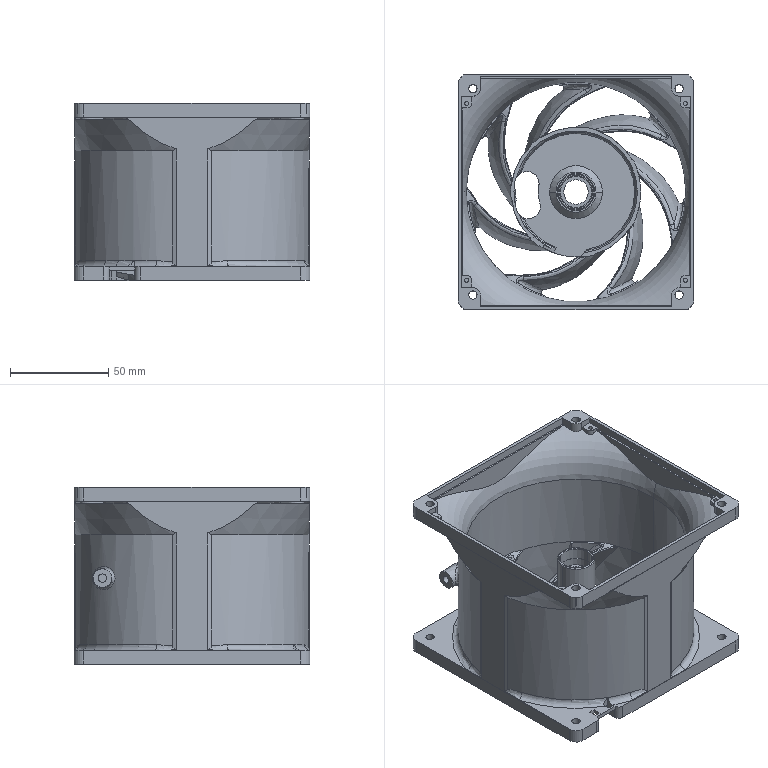NC program | NX | posted with a generic post | part box 120 x 120 x 90.2 mm
Lines 89761 to 90543 of 941997:
(QUICK_ROUGHING , TOOL : D8开粗刀)
N179490 T03 M6
N179492 G54
N179494 G17 G0 G90 X-40.033 Y2.81 S6800 M3
N179496 G43 Z3.6 H3
N179498 Z-0.8
N179500 G94 G1 Z-1.3 F2500.
N179502 G3 X-36.653 Y5.989 R4.
N179504 G2 X-34.912 Y12.669 R43.674
N179506 G3 X-34.604 Y14.896 R51.775
N179508 G2 X-33.059 Y17.237 R5.097
N179510 G3 X-32.058 Y18.68 R7.307
N179512 G1 X-30.488 Y21.219
N179514 G2 X-24.92 Y27.542 R44.968
N179516 X-18.509 Y32.196 R43.58
N179518 X-11.865 Y35.2 R44.159
N179520 G3 X-10.38 Y36.109 R8.325
N179522 G2 X-7.101 Y36.597 R4.998
N179524 G3 X-3.264 Y36.97 R28.124
N179526 X-2.561 Y38.44 R0.967
N179528 G1 X-3.523 Y39.986
N179530 Z-0.8
N179532 G0 Z0.7
N179534 X-3.52 Z0.77
N179536 X-3.511 Z0.839
N179538 X-3.496 Y39.987 Z0.907
N179540 X-3.475 Y39.988 Z0.974
N179542 X-3.449 Y39.989 Z1.038
N179544 X-3.416 Y39.99 Z1.1
N179546 X-3.379 Y39.992 Z1.159
N179548 X-3.336 Y39.994 Z1.214
N179550 X-3.289 Y39.996 Z1.266
N179552 X-3.238 Y39.998 Z1.313
N179554 X-3.183 Y40. Z1.355
N179556 X-3.124 Y40.003 Z1.393
N179558 X-3.062 Y40.005 Z1.425
N179560 X-2.997 Y40.008 Z1.452
N179562 X-2.931 Y40.011 Z1.473
N179564 X-2.863 Y40.014 Z1.488
N179566 X-2.794 Y40.016 Z1.497
N179568 X-2.724 Y40.019 Z1.5
N179570 X-0.994 Y40.092
N179572 X-0.925 Y40.095 Z1.497
N179574 X-0.856 Y40.098 Z1.488
N179576 X-0.787 Y40.101 Z1.473
N179578 X-0.721 Y40.104 Z1.452
N179580 X-0.657 Y40.106 Z1.425
N179582 X-0.595 Y40.109 Z1.393
N179584 X-0.536 Y40.111 Z1.355
N179586 X-0.481 Y40.114 Z1.313
N179588 X-0.429 Y40.116 Z1.266
N179590 X-0.382 Y40.118 Z1.214
N179592 X-0.34 Y40.12 Z1.159
N179594 X-0.302 Y40.121 Z1.1
N179596 X-0.27 Y40.123 Z1.038
N179598 X-0.243 Y40.124 Z0.974
N179600 X-0.222 Y40.125 Z0.907
N179602 X-0.207 Z0.839
N179604 X-0.198 Y40.126 Z0.77
N179606 X-0.195 Z0.7
N179608 Z-0.8
N179610 G1 Z-1.3
N179612 G3 X3.232 Y36.973 R4.
N179614 G2 X19.426 Y31.636 R37.113
N179616 G3 X21.232 Y30.792 R5.732
N179618 G2 X23.894 Y28.827 R4.47
N179620 G3 X25.83 Y26.638 R15.265
N179622 G2 X32.163 Y18.509 R36.014
N179624 G1 X32.706 Y17.606
N179626 X34.407 Y13.993
N179628 G2 X36.951 Y3.715 R41.082
N179630 G3 X37.49 Y2.165 R7.171
N179632 G2 X37.271 Y-1.201 R5.018
N179634 G3 X36.981 Y-3.168 R9.676
N179636 G2 X32.669 Y-17.62 R37.115
N179638 X25.935 Y-26.599 R38.992
N179640 G1 X24.695 Y-28.458
N179642 G2 X22.235 Y-29.913 R5.67
N179644 G3 X20.329 Y-31.043 R16.913
N179646 G2 X14.91 Y-33.978 R31.887
N179648 X13.103 Y-34.723 R10.108
N179650 X6.324 Y-36.587 R39.685
N179652 X-4.182 Y-36.893 R38.958
N179654 G3 X-6.767 Y-37.051 R16.229
N179656 G2 X-9.477 Y-36.037 R5.102
N179658 G1 X-9.735 Y-35.926
N179660 G3 X-11.169 Y-36.84 R1.026
N179662 G1 X-11.214 Y-38.581
N179664 Z-0.8
N179666 G0 Z-0.1
N179668 X-11.211 Y-38.583 Z-0.03
N179670 X-11.204 Y-38.588 Z0.039
N179672 X-11.191 Y-38.596 Z0.107
N179674 X-11.173 Y-38.607 Z0.174
N179676 X-11.151 Y-38.622 Z0.238
N179678 X-11.123 Y-38.639 Z0.3
N179680 X-11.092 Y-38.659 Z0.359
N179682 X-11.056 Y-38.682 Z0.414
N179684 X-11.016 Y-38.707 Z0.466
N179686 X-10.973 Y-38.734 Z0.513
N179688 X-10.926 Y-38.764 Z0.555
N179690 X-10.876 Y-38.796 Z0.593
N179692 X-10.824 Y-38.829 Z0.625
N179694 X-10.769 Y-38.863 Z0.652
N179696 X-10.713 Y-38.899 Z0.673
N179698 X-10.656 Y-38.935 Z0.688
N179700 X-10.597 Y-38.973 Z0.697
N179702 X-10.538 Y-39.01 Z0.7
N179704 X-1.277 Y-44.885
N179706 X-1.218 Y-44.922 Z0.697
N179708 X-1.159 Y-44.959 Z0.688
N179710 X-1.102 Y-44.996 Z0.673
N179712 X-1.046 Y-45.032 Z0.652
N179714 X-0.991 Y-45.066 Z0.625
N179716 X-0.939 Y-45.099 Z0.593
N179718 X-0.889 Y-45.131 Z0.555
N179720 X-0.842 Y-45.16 Z0.513
N179722 X-0.799 Y-45.188 Z0.466
N179724 X-0.759 Y-45.213 Z0.414
N179726 X-0.723 Y-45.236 Z0.359
N179728 X-0.692 Y-45.256 Z0.3
N179730 X-0.664 Y-45.273 Z0.238
N179732 X-0.642 Y-45.288 Z0.174
N179734 X-0.624 Y-45.299 Z0.107
N179736 X-0.611 Y-45.307 Z0.039
N179738 X-0.604 Y-45.312 Z-0.03
N179740 X-0.601 Y-45.314 Z-0.1
N179742 Z-1.6
N179744 G1 Z-2.1
N179746 G2 X1.532 Y-42.648 R4.
N179748 G3 X3.574 Y-41.161 R9.885
N179750 G2 X4.475 Y-40.84 R2.049
N179752 G1 X5.731 Y-40.696
N179754 G2 X7.956 Y-42.7 R1.998
N179756 G1 Z-1.6
N179758 G0 X7.959 Y-42.698 Z-1.53
N179760 X7.967 Y-42.693 Z-1.461
N179762 X7.98 Y-42.686 Z-1.393
N179764 X7.998 Y-42.675 Z-1.326
N179766 X8.021 Y-42.662 Z-1.262
N179768 X8.048 Y-42.645 Z-1.2
N179770 X8.081 Y-42.626 Z-1.141
N179772 X8.117 Y-42.605 Z-1.086
N179774 X8.158 Y-42.581 Z-1.034
N179776 X8.202 Y-42.555 Z-0.987
N179778 X8.25 Y-42.527 Z-0.945
N179780 X8.301 Y-42.497 Z-0.907
N179782 X8.354 Y-42.465 Z-0.875
N179784 X8.41 Y-42.433 Z-0.848
N179786 X8.467 Y-42.399 Z-0.827
N179788 X8.526 Y-42.364 Z-0.812
N179790 X8.586 Y-42.329 Z-0.803
N179792 X8.646 Y-42.294 Z-0.8
N179794 X25.242 Y-32.533
N179796 X25.302 Y-32.498 Z-0.803
N179798 X25.362 Y-32.463 Z-0.812
N179800 X25.42 Y-32.428 Z-0.827
N179802 X25.478 Y-32.394 Z-0.848
N179804 X25.533 Y-32.362 Z-0.875
N179806 X25.587 Y-32.33 Z-0.907
N179808 X25.637 Y-32.301 Z-0.945
N179810 X25.685 Y-32.273 Z-0.987
N179812 X25.73 Y-32.246 Z-1.034
N179814 X25.77 Y-32.223 Z-1.086
N179816 X25.807 Y-32.201 Z-1.141
N179818 X25.839 Y-32.182 Z-1.2
N179820 X25.867 Y-32.166 Z-1.262
N179822 X25.89 Y-32.152 Z-1.326
N179824 X25.908 Y-32.141 Z-1.393
N179826 X25.921 Y-32.134 Z-1.461
N179828 X25.929 Y-32.129 Z-1.53
N179830 X25.932 Y-32.128 Z-1.6
N179832 G1 Z-2.1
N179834 G3 X20.48 Y-30.949 R4.
N179836 G1 X17.62 Y-32.699
N179838 X14.007 Y-34.402
N179840 G2 X5.878 Y-36.676 R43.391
N179842 G3 X1.968 Y-37.13 R56.548
N179844 X1.172 Y-37.742 R1.737
N179846 G2 X-1.348 Y-39.543 R4.107
N179848 X-5.71 Y-38.922 R4.778
N179850 G3 X-7.2 Y-39.648 R0.99
N179852 G1 X-7.425 Y-41.417
N179854 Z-1.6
N179856 G0 Z0.7
N179858 X-7.428 Y-41.416 Z0.77
N179860 X-7.436 Y-41.411 Z0.839
N179862 X-7.448 Y-41.402 Z0.907
N179864 X-7.466 Y-41.391 Z0.974
N179866 X-7.488 Y-41.377 Z1.038
N179868 X-7.515 Y-41.359 Z1.1
N179870 X-7.547 Y-41.339 Z1.159
N179872 X-7.583 Y-41.316 Z1.214
N179874 X-7.623 Y-41.291 Z1.266
N179876 X-7.666 Y-41.263 Z1.313
N179878 X-7.712 Y-41.233 Z1.355
N179880 X-7.762 Y-41.201 Z1.393
N179882 X-7.814 Y-41.168 Z1.425
N179884 X-7.868 Y-41.133 Z1.452
N179886 X-7.924 Y-41.097 Z1.473
N179888 X-7.982 Y-41.06 Z1.488
N179890 X-8.04 Y-41.023 Z1.497
N179892 X-8.099 Y-40.985 Z1.5
N179894 X-11.885 Y-38.557
N179896 X-11.944 Y-38.52 Z1.497
N179898 X-12.002 Y-38.482 Z1.488
N179900 X-12.06 Y-38.445 Z1.473
N179902 X-12.116 Y-38.409 Z1.452
N179904 X-12.17 Y-38.375 Z1.425
N179906 X-12.222 Y-38.341 Z1.393
N179908 X-12.272 Y-38.309 Z1.355
N179910 X-12.318 Y-38.28 Z1.313
N179912 X-12.362 Y-38.252 Z1.266
N179914 X-12.401 Y-38.226 Z1.214
N179916 X-12.437 Y-38.203 Z1.159
N179918 X-12.469 Y-38.183 Z1.1
N179920 X-12.496 Y-38.166 Z1.038
N179922 X-12.518 Y-38.151 Z0.974
N179924 X-12.536 Y-38.14 Z0.907
N179926 X-12.549 Y-38.132 Z0.839
N179928 X-12.556 Y-38.127 Z0.77
N179930 X-12.559 Y-38.125 Z0.7
N179932 Z-0.8
N179934 G1 Z-1.3
N179936 G3 X-14.825 Y-34.015 R4.
N179938 G2 X-18.659 Y-32.071 R29.796
N179940 X-23.929 Y-28.374 R35.194
N179942 X-31.503 Y-19.655 R37.735
N179944 G3 X-32.961 Y-18.09 R7.299
N179946 G2 X-34.078 Y-15.232 R4.788
N179948 G3 X-34.647 Y-13.271 R8.83
N179950 G2 X-36.957 Y-3.368 R35.846
N179952 G3 X-38.424 Y-2.67 R0.963
N179954 G1 X-39.972 Y-3.639
N179956 Z-0.8
N179958 G0 Z-0.1
N179960 X-39.973 Y-3.637 Z-0.03
N179962 X-39.978 Y-3.629 Z0.039
N179964 X-39.985 Y-3.615 Z0.107
N179966 X-39.995 Y-3.597 Z0.174
N179968 X-40.009 Y-3.574 Z0.238
N179970 X-40.025 Y-3.546 Z0.3
N179972 X-40.043 Y-3.513 Z0.359
N179974 X-40.064 Y-3.476 Z0.414
N179976 X-40.087 Y-3.435 Z0.466
N179978 X-40.113 Y-3.391 Z0.513
N179980 X-40.14 Y-3.343 Z0.555
N179982 X-40.169 Y-3.291 Z0.593
N179984 X-40.2 Y-3.238 Z0.625
N179986 X-40.232 Y-3.182 Z0.652
N179988 X-40.265 Y-3.124 Z0.673
N179990 X-40.298 Y-3.065 Z0.688
N179992 X-40.332 Y-3.004 Z0.697
N179994 X-40.367 Y-2.944 Z0.7
N179996 X-42.04 Y-0.001
N179998 X-42.075 Y0.06 Z0.697
N180000 X-42.109 Y0.12 Z0.688
N180002 X-42.142 Y0.179 Z0.673
N180004 X-42.175 Y0.237 Z0.652
N180006 X-42.207 Y0.293 Z0.625
N180008 X-42.238 Y0.347 Z0.593
N180010 X-42.267 Y0.398 Z0.555
N180012 X-42.294 Y0.446 Z0.513
N180014 X-42.32 Y0.491 Z0.466
N180016 X-42.343 Y0.532 Z0.414
N180018 X-42.364 Y0.569 Z0.359
N180020 X-42.383 Y0.601 Z0.3
N180022 X-42.399 Y0.629 Z0.238
N180024 X-42.412 Y0.652 Z0.174
N180026 X-42.422 Y0.671 Z0.107
N180028 X-42.43 Y0.684 Z0.039
N180030 X-42.434 Y0.692 Z-0.03
N180032 X-42.436 Y0.694 Z-0.1
N180034 Z-1.6
N180036 G1 Z-2.1
N180038 G3 X-40.949 Y3.424 R4.
N180040 X-40.868 Y5.466 R7.112
N180042 X-41.624 Y7.158 R24.03
N180044 G1 X-41.917 Y8.015
N180046 G3 X-44.85 Y8.618 R1.733
N180048 G2 X-45.422 Y8.249 R1.068
N180050 X-45.389 Y8.753 R0.531
N180052 X-42.313 Y14.072 R28.836
N180054 X-38.596 Y18.485 R25.146
N180056 X-36.867 Y19.406 R3.238
N180058 X-36.002 Y18.772 R0.918
N180060 X-36.756 Y14.155 R4.
N180062 G3 X-38.26 Y10.38 R4.599
N180064 X-37.455 Y7.671 R4.506
N180066 G2 X-36.631 Y6.282 R1.957
N180068 G3 X-37.071 Y-2.265 R44.612
N180070 G1 X-36.514 Y-6.781
N180072 X-35.854 Y-9.557
N180074 G2 X-36.983 Y-10.706 R0.952
N180076 G1 X-38.785 Y-10.313
N180078 Z-1.6
N180080 G0 Z0.198
N180082 Y-10.315 Z0.242
N180084 X-38.783 Y-10.32 Z0.285
N180086 X-38.781 Y-10.329 Z0.328
N180088 X-38.777 Y-10.342 Z0.37
N180090 X-38.773 Y-10.358 Z0.41
N180092 X-38.767 Y-10.378 Z0.449
N180094 X-38.761 Y-10.4 Z0.486
N180096 X-38.754 Y-10.426 Z0.521
N180098 X-38.746 Y-10.455 Z0.553
N180100 X-38.737 Y-10.486 Z0.583
N180102 X-38.728 Y-10.519 Z0.609
N180104 X-38.718 Y-10.555 Z0.633
N180106 X-38.707 Y-10.592 Z0.653
N180108 X-38.697 Y-10.631 Z0.67
N180110 X-38.685 Y-10.671 Z0.683
N180112 X-38.674 Y-10.713 Z0.692
N180114 X-38.662 Y-10.754 Z0.698
N180116 X-38.65 Y-10.797 Z0.7
N180118 X-38.639 Y-10.839 Z0.698
N180120 X-38.627 Y-10.881 Z0.692
N180122 X-38.615 Y-10.922 Z0.683
N180124 X-38.604 Y-10.962 Z0.67
N180126 X-38.593 Y-11.001 Z0.653
N180128 X-38.583 Y-11.038 Z0.633
N180130 X-38.573 Y-11.074 Z0.609
N180132 X-38.564 Y-11.107 Z0.583
N180134 X-38.555 Y-11.139 Z0.553
N180136 X-38.547 Y-11.167 Z0.521
N180138 X-38.54 Y-11.193 Z0.486
N180140 X-38.534 Y-11.215 Z0.449
N180142 X-38.528 Y-11.235 Z0.41
N180144 X-38.524 Y-11.251 Z0.37
N180146 X-38.52 Y-11.264 Z0.328
N180148 X-38.517 Y-11.273 Z0.285
N180150 X-38.516 Y-11.278 Z0.242
N180152 X-38.515 Y-11.28 Z0.198
N180154 Z-1.6
N180156 G1 Z-2.1
N180158 G2 X-34.369 Y-14.072 R4.
N180160 G1 X-34.123 Y-14.856
N180162 X-34.118 Y-14.889
N180164 X-34.107 Y-15.209
N180166 G2 X-35.483 Y-16.207 R1.025
N180168 G1 X-37.121 Y-15.609
N180170 Z-1.6
N180172 G0 Z-0.1
N180174 X-37.12 Y-15.612 Z-0.03
N180176 X-37.119 Y-15.621 Z0.039
N180178 X-37.118 Y-15.636 Z0.107
N180180 X-37.115 Y-15.657 Z0.174
N180182 X-37.112 Y-15.683 Z0.238
N180184 X-37.109 Y-15.715 Z0.3
N180186 X-37.105 Y-15.752 Z0.359
N180188 X-37.1 Y-15.795 Z0.414
N180190 X-37.095 Y-15.841 Z0.466
N180192 X-37.089 Y-15.893 Z0.513
N180194 X-37.083 Y-15.948 Z0.555
N180196 X-37.077 Y-16.006 Z0.593
N180198 X-37.07 Y-16.068 Z0.625
N180200 X-37.063 Y-16.132 Z0.652
N180202 X-37.055 Y-16.198 Z0.673
N180204 X-37.048 Y-16.266 Z0.688
N180206 X-37.04 Y-16.334 Z0.697
N180208 X-37.032 Y-16.404 Z0.7
N180210 X-35.836 Y-27.164
N180212 X-35.828 Y-27.233 Z0.697
N180214 X-35.821 Y-27.302 Z0.688
N180216 X-35.813 Y-27.37 Z0.673
N180218 X-35.806 Y-27.436 Z0.652
N180220 X-35.799 Y-27.5 Z0.625
N180222 X-35.792 Y-27.562 Z0.593
N180224 X-35.785 Y-27.62 Z0.555
N180226 X-35.779 Y-27.675 Z0.513
N180228 X-35.774 Y-27.726 Z0.466
N180230 X-35.768 Y-27.773 Z0.414
N180232 X-35.764 Y-27.815 Z0.359
N180234 X-35.76 Y-27.853 Z0.3
N180236 X-35.756 Y-27.885 Z0.238
N180238 X-35.753 Y-27.911 Z0.174
N180240 X-35.751 Y-27.932 Z0.107
N180242 X-35.749 Y-27.947 Z0.039
N180244 X-35.748 Y-27.956 Z-0.03
N180246 Y-27.959 Z-0.1
N180248 Z-1.6
N180250 G1 Z-2.1
N180252 G2 X-32.426 Y-27.805 R4.
N180254 G3 X-29.971 Y-28.46 R9.582
N180256 G2 X-29.058 Y-29.008 R2.142
N180258 G1 X-28.16 Y-29.903
N180260 G2 X-27.746 Y-32.869 R2.48
N180262 G1 Z-1.6
N180264 G0 X-27.743 Y-32.87 Z-1.53
N180266 X-27.734 Y-32.873 Z-1.461
N180268 X-27.72 Y-32.878 Z-1.393
N180270 X-27.7 Y-32.885 Z-1.326
N180272 X-27.675 Y-32.894 Z-1.262
N180274 X-27.645 Y-32.904 Z-1.2
N180276 X-27.609 Y-32.917 Z-1.141
N180278 X-27.569 Y-32.93 Z-1.086
N180280 X-27.524 Y-32.946 Z-1.034
N180282 X-27.476 Y-32.963 Z-0.987
N180284 X-27.424 Y-32.981 Z-0.945
N180286 X-27.368 Y-33. Z-0.907
N180288 X-27.309 Y-33.02 Z-0.875
N180290 X-27.248 Y-33.041 Z-0.848
N180292 X-27.186 Y-33.063 Z-0.827
N180294 X-27.121 Y-33.085 Z-0.812
N180296 X-27.056 Y-33.108 Z-0.803
N180298 X-26.99 Y-33.131 Z-0.8
N180300 X-13.301 Y-37.868
N180302 X-13.235 Y-37.891 Z-0.803
N180304 X-13.169 Y-37.914 Z-0.812
N180306 X-13.105 Y-37.936 Z-0.827
N180308 X-13.042 Y-37.958 Z-0.848
N180310 X-12.981 Y-37.979 Z-0.875
N180312 X-12.923 Y-37.999 Z-0.907
N180314 X-12.867 Y-38.019 Z-0.945
N180316 X-12.815 Y-38.037 Z-0.987
N180318 X-12.766 Y-38.054 Z-1.034
N180320 X-12.722 Y-38.069 Z-1.086
N180322 X-12.681 Y-38.083 Z-1.141
N180324 X-12.646 Y-38.095 Z-1.2
N180326 X-12.616 Y-38.106 Z-1.262
N180328 X-12.59 Y-38.114 Z-1.326
N180330 X-12.57 Y-38.121 Z-1.393
N180332 X-12.556 Y-38.126 Z-1.461
N180334 X-12.548 Y-38.129 Z-1.53
N180336 X-12.545 Y-38.13 Z-1.6
N180338 G1 Z-2.1
N180340 G3 X-14.811 Y-34.022 R4.
N180342 G2 X-18.659 Y-32.071 R30.072
N180344 X-23.929 Y-28.374 R35.215
N180346 X-27.685 Y-24.794 R53.722
N180348 G3 X-28.777 Y-24.459 R1.484
N180350 G2 X-31.258 Y-23.942 R4.064
N180352 X-32.961 Y-22.556 R7.072
N180354 X-33.994 Y-19.684 R5.157
N180356 G3 X-35.49 Y-18.963 R0.993
N180358 G1 X-37.015 Y-19.879
N180360 Z-1.6
N180362 G0 Z-0.487
N180364 Y-19.877 Z-0.454
N180366 X-37.016 Y-19.873 Z-0.42
N180368 Y-19.866 Z-0.387
N180370 Y-19.855 Z-0.355
N180372 X-37.017 Y-19.843 Z-0.324
N180374 X-37.018 Y-19.827 Z-0.294
N180376 X-37.019 Y-19.809 Z-0.265
N180378 X-37.02 Y-19.788 Z-0.238
N180380 X-37.022 Y-19.765 Z-0.213
N180382 X-37.023 Y-19.741 Z-0.191
N180384 X-37.024 Y-19.714 Z-0.17
N180386 X-37.026 Y-19.685 Z-0.152
N180388 X-37.028 Y-19.655 Z-0.136
N180390 X-37.029 Y-19.624 Z-0.123
N180392 X-37.031 Y-19.592 Z-0.113
N180394 X-37.033 Y-19.559 Z-0.106
N180396 X-37.035 Y-19.526 Z-0.101
N180398 X-37.037 Y-19.492 Z-0.1
N180400 X-37.039 Y-19.458 Z-0.101
N180402 X-37.041 Y-19.425 Z-0.106
N180404 X-37.042 Y-19.392 Z-0.113
N180406 X-37.044 Y-19.36 Z-0.123
N180408 X-37.046 Y-19.329 Z-0.136
N180410 X-37.048 Y-19.299 Z-0.152
N180412 X-37.049 Y-19.27 Z-0.17
N180414 X-37.051 Y-19.243 Z-0.191
N180416 X-37.052 Y-19.219 Z-0.213
N180418 X-37.053 Y-19.196 Z-0.238
N180420 X-37.054 Y-19.175 Z-0.265
N180422 X-37.055 Y-19.157 Z-0.294
N180424 X-37.056 Y-19.142 Z-0.324
N180426 X-37.057 Y-19.129 Z-0.355
N180428 X-37.058 Y-19.118 Z-0.387
N180430 Y-19.111 Z-0.42
N180432 Y-19.107 Z-0.454
N180434 Y-19.105 Z-0.487
N180436 Z-2.4
N180438 G1 Z-2.9
N180440 G3 X-34.107 Y-15.21 R4.
N180442 X-34.368 Y-14.076 R3.165
N180444 X-35.989 Y-13.652 R1.005
N180446 G1 X-37.302 Y-14.824
N180448 Z-2.4
N180450 G0 Z-0.59
N180452 X-37.303 Y-14.822 Z-0.547
N180454 X-37.305 Y-14.817 Z-0.505
N180456 X-37.308 Y-14.808 Z-0.463
N180458 X-37.313 Y-14.796 Z-0.422
N180460 X-37.319 Y-14.781 Z-0.383
N180462 X-37.326 Y-14.763 Z-0.345
N180464 X-37.334 Y-14.741 Z-0.309
N180466 X-37.344 Y-14.717 Z-0.275
N180468 X-37.354 Y-14.69 Z-0.244
N180470 X-37.365 Y-14.661 Z-0.215
N180472 X-37.377 Y-14.629 Z-0.189
N180474 X-37.39 Y-14.595 Z-0.166
N180476 X-37.404 Y-14.56 Z-0.146
N180478 X-37.418 Y-14.523 Z-0.13
N180480 X-37.433 Y-14.485 Z-0.117
N180482 X-37.448 Y-14.446 Z-0.107
N180484 X-37.463 Y-14.406 Z-0.102
N180486 X-37.478 Y-14.367 Z-0.1
N180488 X-37.493 Y-14.327 Z-0.102
N180490 X-37.509 Y-14.287 Z-0.107
N180492 X-37.523 Y-14.248 Z-0.117
N180494 X-37.538 Y-14.21 Z-0.13
N180496 X-37.552 Y-14.173 Z-0.146
N180498 X-37.566 Y-14.138 Z-0.166
N180500 X-37.579 Y-14.104 Z-0.189
N180502 X-37.591 Y-14.072 Z-0.215
N180504 X-37.602 Y-14.043 Z-0.244
N180506 X-37.613 Y-14.016 Z-0.275
N180508 X-37.622 Y-13.992 Z-0.309
N180510 X-37.63 Y-13.97 Z-0.345
N180512 X-37.637 Y-13.952 Z-0.383
N180514 X-37.643 Y-13.937 Z-0.422
N180516 X-37.648 Y-13.925 Z-0.463
N180518 X-37.651 Y-13.916 Z-0.505
N180520 X-37.653 Y-13.911 Z-0.547
N180522 X-37.654 Y-13.909 Z-0.59
N180524 Z-2.4
N180526 G1 Z-2.9
N180528 G3 X-35.85 Y-9.572 R4.
N180530 G2 X-36.982 Y-3.168 R35.604
N180532 X-37.095 Y1.921 R44.27
N180534 G3 X-37.85 Y2.62 R0.725
N180536 G2 X-41.532 Y5.864 R3.919
N180538 X-41.519 Y8.574 R6.671
N180540 X-40.556 Y10.399 R5.255
N180542 G3 X-41.036 Y11.943 R0.956
N180544 G1 X-42.812 Y12.419
N180546 Z-2.4
N180548 G0 Z-1.7
N180550 X-42.814 Y12.416 Z-1.63
N180552 X-42.82 Y12.41 Z-1.561
N180554 X-42.83 Y12.398 Z-1.493
N180556 X-42.844 Y12.383 Z-1.426
N180558 X-42.862 Y12.363 Z-1.362
N180560 X-42.883 Y12.339 Z-1.3
N180562 X-42.908 Y12.311 Z-1.241
N180564 X-42.937 Y12.279 Z-1.186
N180566 X-42.968 Y12.244 Z-1.134
N180568 X-43.002 Y12.206 Z-1.087
N180570 X-43.039 Y12.165 Z-1.045
N180572 X-43.079 Y12.121 Z-1.007
N180574 X-43.12 Y12.075 Z-0.975
N180576 X-43.163 Y12.027 Z-0.948
N180578 X-43.208 Y11.977 Z-0.927
N180580 X-43.253 Y11.926 Z-0.912
N180582 X-43.299 Y11.875 Z-0.903
N180584 X-43.346 Y11.823 Z-0.9
N180586 X-43.602 Y11.537
N180588 X-43.649 Y11.485 Z-0.903
N180590 X-43.695 Y11.434 Z-0.912
N180592 X-43.74 Y11.383 Z-0.927
N180594 X-43.785 Y11.333 Z-0.948
N180596 X-43.828 Y11.285 Z-0.975
N180598 X-43.869 Y11.239 Z-1.007
N180600 X-43.908 Y11.196 Z-1.045
N180602 X-43.945 Y11.154 Z-1.087
N180604 X-43.98 Y11.116 Z-1.134
N180606 X-44.011 Y11.081 Z-1.186
N180608 X-44.039 Y11.049 Z-1.241
N180610 X-44.064 Y11.021 Z-1.3
N180612 X-44.086 Y10.997 Z-1.362
N180614 X-44.104 Y10.977 Z-1.426
N180616 X-44.118 Y10.962 Z-1.493
N180618 X-44.128 Y10.951 Z-1.561
N180620 X-44.134 Y10.944 Z-1.63
N180622 X-44.136 Y10.942 Z-1.7
N180624 Z-3.2
N180626 G1 Z-3.7
N180628 G2 X-43.917 Y6.423 R4.
N180630 G3 X-44.813 Y3.155 R4.897
N180632 X-43.799 Y0.132 R4.857
N180634 X-39.283 Y-1.008 R4.033
N180636 X-37.486 Y0.241 R5.069
N180638 G2 X-37.124 Y0.157 R0.198
N180640 G1 X-37.072 Y-2.265
N180642 X-36.514 Y-6.781
N180644 X-35.847 Y-9.587
N180646 G2 X-36.976 Y-10.737 R0.952
N180648 G1 X-38.778 Y-10.344
N180650 Z-3.2
N180652 G0 Z-1.388
N180654 Y-10.346 Z-1.346
N180656 X-38.776 Y-10.351 Z-1.304
N180658 X-38.774 Y-10.36 Z-1.262
N180660 X-38.77 Y-10.372 Z-1.221
N180662 X-38.766 Y-10.388 Z-1.182
N180664 X-38.76 Y-10.407 Z-1.144
N180666 X-38.754 Y-10.429 Z-1.108
N180668 X-38.747 Y-10.454 Z-1.074
N180670 X-38.739 Y-10.482 Z-1.043
N180672 X-38.731 Y-10.512 Z-1.014
N180674 X-38.722 Y-10.545 Z-0.988
N180676 X-38.712 Y-10.579 Z-0.965
N180678 X-38.702 Y-10.616 Z-0.946
N180680 X-38.691 Y-10.654 Z-0.929
N180682 X-38.68 Y-10.693 Z-0.917
N180684 X-38.669 Y-10.733 Z-0.907
N180686 X-38.658 Y-10.773 Z-0.902
N180688 X-38.646 Y-10.814 Z-0.9
N180690 X-38.635 Y-10.855 Z-0.902
N180692 X-38.624 Y-10.896 Z-0.907
N180694 X-38.612 Y-10.936 Z-0.917
N180696 X-38.601 Y-10.975 Z-0.929
N180698 X-38.591 Y-11.013 Z-0.946
N180700 X-38.581 Y-11.05 Z-0.965
N180702 X-38.571 Y-11.084 Z-0.988
N180704 X-38.562 Y-11.117 Z-1.014
N180706 X-38.553 Y-11.147 Z-1.043
N180708 X-38.546 Y-11.175 Z-1.074
N180710 X-38.539 Y-11.2 Z-1.108
N180712 X-38.532 Y-11.222 Z-1.144
N180714 X-38.527 Y-11.241 Z-1.182
N180716 X-38.523 Y-11.257 Z-1.221
N180718 X-38.519 Y-11.269 Z-1.262
N180720 X-38.517 Y-11.278 Z-1.304
N180722 X-38.515 Y-11.283 Z-1.346
N180724 Y-11.285 Z-1.388
N180726 Z-3.2
N180728 G1 Z-3.7
N180730 G2 X-34.369 Y-14.075 R4.
N180732 G1 X-34.122 Y-14.862
N180734 X-34.117 Y-14.894
N180736 X-34.107 Y-15.212
N180738 G2 X-35.485 Y-16.208 R1.026
N180740 G1 X-37.121 Y-15.609
N180742 Z-3.2
N180744 G0 Z-2.5
N180746 Y-15.612 Z-2.43
N180748 Y-15.621 Z-2.361
N180750 Y-15.637 Z-2.293
N180752 Y-15.658 Z-2.226
N180754 X-37.12 Y-15.684 Z-2.162
N180756 X-37.119 Y-15.716 Z-2.1
N180758 Y-15.754 Z-2.041
N180760 X-37.118 Y-15.796 Z-1.986
N180762 X-37.117 Y-15.844 Z-1.934
N180764 X-37.116 Y-15.895 Z-1.887
N180766 X-37.115 Y-15.95 Z-1.845
N180768 X-37.114 Y-16.009 Z-1.807
N180770 X-37.113 Y-16.071 Z-1.775
N180772 X-37.112 Y-16.136 Z-1.748
N180774 X-37.111 Y-16.202 Z-1.727
N180776 X-37.11 Y-16.27 Z-1.712
N180778 X-37.108 Y-16.339 Z-1.703
N180780 X-37.107 Y-16.409 Z-1.7
N180782 X-37.073 Y-18.308
N180784 X-37.072 Y-18.378 Z-1.703
N180786 X-37.071 Y-18.447 Z-1.712
N180788 X-37.07 Y-18.516 Z-1.727
N180790 X-37.068 Y-18.582 Z-1.748
N180792 X-37.067 Y-18.647 Z-1.775
N180794 X-37.066 Y-18.708 Z-1.807
N180796 X-37.065 Y-18.767 Z-1.845
N180798 X-37.064 Y-18.823 Z-1.887
N180800 X-37.063 Y-18.874 Z-1.934
N180802 X-37.062 Y-18.921 Z-1.986
N180804 Y-18.964 Z-2.041
N180806 X-37.061 Y-19.001 Z-2.1
N180808 X-37.06 Y-19.033 Z-2.162
N180810 Y-19.06 Z-2.226
N180812 Y-19.081 Z-2.293
N180814 X-37.059 Y-19.096 Z-2.361
N180816 Y-19.105 Z-2.43
N180818 Y-19.108 Z-2.5
N180820 Z-4.
N180822 G1 Z-4.5
N180824 G3 X-34.107 Y-15.213 R4.
N180826 X-34.37 Y-14.074 R3.157
N180828 X-35.992 Y-13.652 R1.006
N180830 G1 X-37.303 Y-14.825
N180832 Z-4.
N180834 G0 Z-2.175
N180836 X-37.304 Y-14.824 Z-2.134
N180838 X-37.306 Y-14.819 Z-2.093
N180840 X-37.309 Y-14.81 Z-2.052
N180842 X-37.314 Y-14.799 Z-2.013
N180844 X-37.319 Y-14.784 Z-1.975
N180846 X-37.326 Y-14.766 Z-1.938
N180848 X-37.334 Y-14.745 Z-1.903
N180850 X-37.343 Y-14.722 Z-1.87
N180852 X-37.353 Y-14.695 Z-1.839
N180854 X-37.364 Y-14.667 Z-1.811
N180856 X-37.376 Y-14.636 Z-1.786
N180858 X-37.389 Y-14.604 Z-1.764
N180860 X-37.402 Y-14.569 Z-1.745
N180862 X-37.416 Y-14.533 Z-1.729
N180864 X-37.43 Y-14.496 Z-1.716
N180866 X-37.444 Y-14.459 Z-1.707
N180868 X-37.459 Y-14.42 Z-1.702
N180870 X-37.474 Y-14.382 Z-1.7
N180872 X-37.489 Y-14.343 Z-1.702
N180874 X-37.504 Y-14.305 Z-1.707
N180876 X-37.518 Y-14.267 Z-1.716
N180878 X-37.532 Y-14.23 Z-1.729
N180880 X-37.546 Y-14.194 Z-1.745
N180882 X-37.559 Y-14.16 Z-1.764
N180884 X-37.572 Y-14.127 Z-1.786
N180886 X-37.584 Y-14.096 Z-1.811
N180888 X-37.595 Y-14.068 Z-1.839
N180890 X-37.605 Y-14.042 Z-1.87
N180892 X-37.614 Y-14.018 Z-1.903
N180894 X-37.622 Y-13.997 Z-1.938
N180896 X-37.629 Y-13.979 Z-1.975
N180898 X-37.634 Y-13.965 Z-2.013
N180900 X-37.639 Y-13.953 Z-2.052
N180902 X-37.642 Y-13.945 Z-2.093
N180904 X-37.644 Y-13.939 Z-2.134
N180906 X-37.645 Y-13.938 Z-2.175
N180908 Z-4.
N180910 G1 Z-4.5
N180912 G3 X-35.843 Y-9.602 R4.
N180914 G2 X-37.103 Y-0.343 R35.519
N180916 G3 X-37.309 Y-0.097 R0.189
N180918 X-38.169 Y-1.088 R4.306
N180920 G1 X-40.347 Y-4.071
N180922 G2 X-43.799 Y-5.578 R4.403
N180924 X-47.494 Y-2.265 R4.068
N180926 X-47.599 Y0.445 R7.122
N180928 X-46.341 Y3.055 R8.199
N180930 G3 X-46.998 Y4.646 R1.047
N180932 G1 X-48.656 Y5.006
N180934 Z-4.
N180936 G0 Z-2.5
N180938 Y5.009 Z-2.43
N180940 Y5.018 Z-2.361
N180942 X-48.657 Y5.033 Z-2.293
N180944 Y5.054 Z-2.226
N180946 X-48.658 Y5.081 Z-2.162
N180948 X-48.659 Y5.113 Z-2.1
N180950 X-48.66 Y5.15 Z-2.041
N180952 X-48.662 Y5.193 Z-1.986
N180954 X-48.663 Y5.24 Z-1.934
N180956 X-48.665 Y5.291 Z-1.887
N180958 X-48.667 Y5.347 Z-1.845
N180960 X-48.669 Y5.405 Z-1.807
N180962 X-48.671 Y5.467 Z-1.775
N180964 X-48.673 Y5.532 Z-1.748
N180966 X-48.675 Y5.598 Z-1.727
N180968 X-48.678 Y5.666 Z-1.712
N180970 X-48.68 Y5.736 Z-1.703
N180972 X-48.682 Y5.805 Z-1.7
N180974 X-48.752 Y7.916
N180976 X-48.754 Y7.986 Z-1.703
N180978 X-48.756 Y8.055 Z-1.712
N180980 X-48.759 Y8.123 Z-1.727
N180982 X-48.761 Y8.19 Z-1.748
N180984 X-48.763 Y8.254 Z-1.775
N180986 X-48.765 Y8.316 Z-1.807
N180988 X-48.767 Y8.375 Z-1.845
N180990 X-48.769 Y8.43 Z-1.887
N180992 X-48.77 Y8.481 Z-1.934
N180994 X-48.772 Y8.529 Z-1.986
N180996 X-48.773 Y8.571 Z-2.041
N180998 X-48.775 Y8.609 Z-2.1
N181000 X-48.776 Y8.641 Z-2.162
N181002 X-48.777 Y8.667 Z-2.226
N181004 Y8.688 Z-2.293
N181006 X-48.778 Y8.704 Z-2.361
N181008 Y8.713 Z-2.43
N181010 Y8.716 Z-2.5
N181012 Z-4.
N181014 G1 Z-4.5
N181016 G3 X-52.287 Y5.143 R4.
N181018 X-51.293 Y-11.325 R52.273
N181020 X-49.646 Y-12.035 R1.111
N181022 G1 X-48.256 Y-11.216
N181024 Z-4.
N181026 G0 Z-3.3
N181028 X-48.254 Y-11.218 Z-3.23
N181030 X-48.249 Y-11.226 Z-3.161
N181032 X-48.24 Y-11.238 Z-3.093
N181034 X-48.228 Y-11.255 Z-3.026
N181036 X-48.212 Y-11.277 Z-2.962
N181038 X-48.193 Y-11.303 Z-2.9
N181040 X-48.172 Y-11.334 Z-2.841
N181042 X-48.147 Y-11.368 Z-2.786
N181044 X-48.119 Y-11.407 Z-2.734
N181046 X-48.09 Y-11.448 Z-2.687
N181048 X-48.057 Y-11.493 Z-2.645